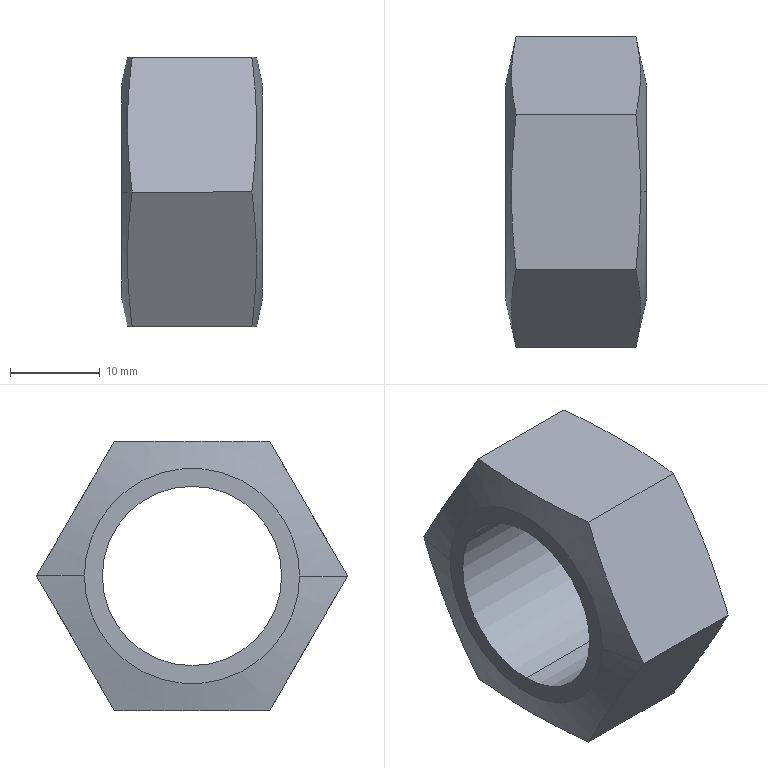Part | SolidWorks | features BaseBody 1 | 1 solid | 14 faces | box 15.7 x 34.641 x 30 mm | volume 7009 mm3 | plane 8 | cone 4 | cylinder 2 | commonest cylinder face diameters 20 x2
STEP:
#1=CARTESIAN_POINT('',(65.7,0.,-10.));
#2=VERTEX_POINT('',#1);
#3=CARTESIAN_POINT('',(65.7,0.,10.));
#4=VERTEX_POINT('',#3);
#5=CARTESIAN_POINT('',(65.7,0.,0.));
#6=DIRECTION('',(-1.,0.,0.));
#7=DIRECTION('',(0.,0.,1.));
#8=AXIS2_PLACEMENT_3D('',#5,#6,#7);
#9=CIRCLE('',#8,10.);
#10=EDGE_CURVE('',#2,#4,#9,.T.);
#11=ORIENTED_EDGE('',*,*,#10,.F.);
#12=CARTESIAN_POINT('',(50.,0.,-10.));
#13=VERTEX_POINT('',#12);
#14=CARTESIAN_POINT('',(50.,0.,-10.));
#15=DIRECTION('',(-1.,0.,0.));
#16=VECTOR('',#15,1000.);
#17=LINE('',#14,#16);
#18=EDGE_CURVE('',#2,#13,#17,.T.);
#19=ORIENTED_EDGE('',*,*,#18,.T.);
#20=CARTESIAN_POINT('',(50.,0.,10.));
#21=VERTEX_POINT('',#20);
#22=CARTESIAN_POINT('',(50.,0.,0.));
#23=DIRECTION('',(1.,0.,0.));
#24=DIRECTION('',(0.,0.,1.));
#25=AXIS2_PLACEMENT_3D('',#22,#23,#24);
#26=CIRCLE('',#25,10.);
#27=EDGE_CURVE('',#21,#13,#26,.T.);
#28=ORIENTED_EDGE('',*,*,#27,.F.);
#29=CARTESIAN_POINT('',(50.,0.,10.));
#30=DIRECTION('',(-1.,0.,0.));
#31=VECTOR('',#30,1000.);
#32=LINE('',#29,#31);
#33=EDGE_CURVE('',#4,#21,#32,.T.);
#34=ORIENTED_EDGE('',*,*,#33,.F.);
#35=EDGE_LOOP('',(#11,#19,#28,#34));
#36=FACE_OUTER_BOUND('',#35,.T.);
#37=CARTESIAN_POINT('',(50.,0.,0.));
#38=DIRECTION('',(-1.,0.,0.));
#39=DIRECTION('',(0.,0.,1.));
#40=AXIS2_PLACEMENT_3D('',#37,#38,#39);
#41=CYLINDRICAL_SURFACE('',#40,10.);
#42=ADVANCED_FACE('',(#36),#41,.F.);
#43=CARTESIAN_POINT('',(65.7,0.,-12.));
#44=VERTEX_POINT('',#43);
#45=CARTESIAN_POINT('',(65.7,0.,12.));
#46=VERTEX_POINT('',#45);
#47=CARTESIAN_POINT('',(65.7,0.,0.));
#48=DIRECTION('',(1.,0.,0.));
#49=DIRECTION('',(0.,0.,1.));
#50=AXIS2_PLACEMENT_3D('',#47,#48,#49);
#51=CIRCLE('',#50,12.);
#52=EDGE_CURVE('',#44,#46,#51,.T.);
#53=ORIENTED_EDGE('',*,*,#52,.F.);
#54=CARTESIAN_POINT('',(65.033,0.,-15.));
#55=VERTEX_POINT('',#54);
#56=CARTESIAN_POINT('',(64.511,0.,-17.352));
#57=DIRECTION('',(-0.2169,0.,-0.9762));
#58=VECTOR('',#57,1000.);
#59=LINE('',#56,#58);
#60=EDGE_CURVE('',#44,#55,#59,.T.);
#61=ORIENTED_EDGE('',*,*,#60,.T.);
#62=CARTESIAN_POINT('',(64.518,8.66,-15.));
#63=VERTEX_POINT('',#62);
#64=CARTESIAN_POINT('',(65.033,0.,-15.));
#65=CARTESIAN_POINT('',(65.033,1.448,-15.));
#66=CARTESIAN_POINT('',(64.986,2.894,-15.));
#67=CARTESIAN_POINT('',(64.808,5.781,-15.));
#68=CARTESIAN_POINT('',(64.678,7.221,-15.));
#69=CARTESIAN_POINT('',(64.518,8.66,-15.));
#70=B_SPLINE_CURVE_WITH_KNOTS('',3,(#64,#65,#66,#67,#68,#69),.UNSPECIFIED.,.F.,.F.,(4,2,4),(0.,0.004338,0.008676),.UNSPECIFIED.);
#71=EDGE_CURVE('',#55,#63,#70,.T.);
#72=ORIENTED_EDGE('',*,*,#71,.T.);
#73=CARTESIAN_POINT('',(64.518,17.321,-0.00000001));
#74=VERTEX_POINT('',#73);
#75=CARTESIAN_POINT('',(64.518,8.66,-15.));
#76=CARTESIAN_POINT('',(64.678,9.382,-13.75));
#77=CARTESIAN_POINT('',(64.808,10.104,-12.5));
#78=CARTESIAN_POINT('',(64.986,11.547,-10.));
#79=CARTESIAN_POINT('',(65.08,12.99,-7.5));
#80=CARTESIAN_POINT('',(64.986,14.434,-5.));
#81=CARTESIAN_POINT('',(64.808,15.877,-2.5));
#82=CARTESIAN_POINT('',(64.678,16.599,-1.25));
#83=CARTESIAN_POINT('',(64.518,17.321,-0.00000001));
#84=B_SPLINE_CURVE_WITH_KNOTS('',3,(#75,#76,#77,#78,#79,#80,#81,#82,#83),.UNSPECIFIED.,.F.,.F.,(4,2,1,2,4),(0.,0.00433,0.00866,0.01299,0.01732),.UNSPECIFIED.);
#85=EDGE_CURVE('',#63,#74,#84,.T.);
#86=ORIENTED_EDGE('',*,*,#85,.T.);
#87=CARTESIAN_POINT('',(64.518,8.66,15.));
#88=VERTEX_POINT('',#87);
#89=CARTESIAN_POINT('',(64.518,17.321,-0.00000001));
#90=CARTESIAN_POINT('',(64.678,16.599,1.25));
#91=CARTESIAN_POINT('',(64.808,15.877,2.5));
#92=CARTESIAN_POINT('',(64.986,14.434,5.));
#93=CARTESIAN_POINT('',(65.08,12.99,7.5));
#94=CARTESIAN_POINT('',(64.986,11.547,10.));
#95=CARTESIAN_POINT('',(64.808,10.104,12.5));
#96=CARTESIAN_POINT('',(64.678,9.382,13.75));
#97=CARTESIAN_POINT('',(64.518,8.66,15.));
#98=B_SPLINE_CURVE_WITH_KNOTS('',3,(#89,#90,#91,#92,#93,#94,#95,#96,#97),.UNSPECIFIED.,.F.,.F.,(4,2,1,2,4),(0.,0.00433,0.00866,0.01299,0.01732),.UNSPECIFIED.);
#99=EDGE_CURVE('',#74,#88,#98,.T.);
#100=ORIENTED_EDGE('',*,*,#99,.T.);
#101=CARTESIAN_POINT('',(65.033,0.,15.));
#102=VERTEX_POINT('',#101);
#103=CARTESIAN_POINT('',(64.518,8.66,15.));
#104=CARTESIAN_POINT('',(64.678,7.221,15.));
#105=CARTESIAN_POINT('',(64.808,5.781,15.));
#106=CARTESIAN_POINT('',(64.986,2.894,15.));
#107=CARTESIAN_POINT('',(65.033,1.448,15.));
#108=CARTESIAN_POINT('',(65.033,0.,15.));
#109=B_SPLINE_CURVE_WITH_KNOTS('',3,(#103,#104,#105,#106,#107,#108),.UNSPECIFIED.,.F.,.F.,(4,2,4),(0.,0.004338,0.008676),.UNSPECIFIED.);
#110=EDGE_CURVE('',#88,#102,#109,.T.);
#111=ORIENTED_EDGE('',*,*,#110,.T.);
#112=CARTESIAN_POINT('',(64.511,0.,17.352));
#113=DIRECTION('',(-0.2169,0.,0.9762));
#114=VECTOR('',#113,1000.);
#115=LINE('',#112,#114);
#116=EDGE_CURVE('',#46,#102,#115,.T.);
#117=ORIENTED_EDGE('',*,*,#116,.F.);
#118=EDGE_LOOP('',(#53,#61,#72,#86,#100,#111,#117));
#119=FACE_OUTER_BOUND('',#118,.T.);
#120=CARTESIAN_POINT('',(64.511,0.,0.));
#121=DIRECTION('',(-1.,0.,0.));
#122=DIRECTION('',(0.,0.,1.));
#123=AXIS2_PLACEMENT_3D('',#120,#121,#122);
#124=CONICAL_SURFACE('',#123,17.352,1.352);
#125=ADVANCED_FACE('',(#119),#124,.T.);
#126=CARTESIAN_POINT('',(50.,-12.,0.));
#127=VERTEX_POINT('',#126);
#128=CARTESIAN_POINT('',(50.,12.,0.));
#129=VERTEX_POINT('',#128);
#130=CARTESIAN_POINT('',(50.,0.,0.));
#131=DIRECTION('',(-1.,0.,0.));
#132=DIRECTION('',(0.,1.,0.));
#133=AXIS2_PLACEMENT_3D('',#130,#131,#132);
#134=CIRCLE('',#133,12.);
#135=EDGE_CURVE('',#127,#129,#134,.T.);
#136=ORIENTED_EDGE('',*,*,#135,.F.);
#137=CARTESIAN_POINT('',(51.182,-17.321,-0.000000021));
#138=VERTEX_POINT('',#137);
#139=CARTESIAN_POINT('',(51.189,-17.352,0.));
#140=DIRECTION('',(0.2169,-0.9762,0.));
#141=VECTOR('',#140,1000.);
#142=LINE('',#139,#141);
#143=EDGE_CURVE('',#127,#138,#142,.T.);
#144=ORIENTED_EDGE('',*,*,#143,.T.);
#145=CARTESIAN_POINT('',(51.182,-8.66,15.));
#146=VERTEX_POINT('',#145);
#147=CARTESIAN_POINT('',(51.182,-17.321,-0.000000021));
#148=CARTESIAN_POINT('',(51.022,-16.599,1.25));
#149=CARTESIAN_POINT('',(50.892,-15.877,2.5));
#150=CARTESIAN_POINT('',(50.714,-14.434,5.));
#151=CARTESIAN_POINT('',(50.62,-12.99,7.5));
#152=CARTESIAN_POINT('',(50.714,-11.547,10.));
#153=CARTESIAN_POINT('',(50.892,-10.104,12.5));
#154=CARTESIAN_POINT('',(51.022,-9.382,13.75));
#155=CARTESIAN_POINT('',(51.182,-8.66,15.));
#156=B_SPLINE_CURVE_WITH_KNOTS('',3,(#147,#148,#149,#150,#151,#152,#153,#154,#155),.UNSPECIFIED.,.F.,.F.,(4,2,1,2,4),(0.,0.00433,0.00866,0.01299,0.01732),.UNSPECIFIED.);
#157=EDGE_CURVE('',#138,#146,#156,.T.);
#158=ORIENTED_EDGE('',*,*,#157,.T.);
#159=CARTESIAN_POINT('',(51.182,8.66,15.));
#160=VERTEX_POINT('',#159);
#161=CARTESIAN_POINT('',(51.182,-8.66,15.));
#162=CARTESIAN_POINT('',(51.022,-7.217,15.));
#163=CARTESIAN_POINT('',(50.892,-5.774,15.));
#164=CARTESIAN_POINT('',(50.714,-2.887,15.));
#165=CARTESIAN_POINT('',(50.62,-0.000000031,15.));
#166=CARTESIAN_POINT('',(50.714,2.887,15.));
#167=CARTESIAN_POINT('',(50.892,5.774,15.));
#168=CARTESIAN_POINT('',(51.022,7.217,15.));
#169=CARTESIAN_POINT('',(51.182,8.66,15.));
#170=B_SPLINE_CURVE_WITH_KNOTS('',3,(#161,#162,#163,#164,#165,#166,#167,#168,#169),.UNSPECIFIED.,.F.,.F.,(4,2,1,2,4),(0.,0.00433,0.00866,0.01299,0.01732),.UNSPECIFIED.);
#171=EDGE_CURVE('',#146,#160,#170,.T.);
#172=ORIENTED_EDGE('',*,*,#171,.T.);
#173=CARTESIAN_POINT('',(51.182,17.321,0.000000003));
#174=VERTEX_POINT('',#173);
#175=CARTESIAN_POINT('',(51.182,8.66,15.));
#176=CARTESIAN_POINT('',(51.022,9.382,13.75));
#177=CARTESIAN_POINT('',(50.892,10.104,12.5));
#178=CARTESIAN_POINT('',(50.714,11.547,10.));
#179=CARTESIAN_POINT('',(50.62,12.99,7.5));
#180=CARTESIAN_POINT('',(50.714,14.434,5.));
#181=CARTESIAN_POINT('',(50.892,15.877,2.5));
#182=CARTESIAN_POINT('',(51.022,16.599,1.25));
#183=CARTESIAN_POINT('',(51.182,17.321,0.000000003));
#184=B_SPLINE_CURVE_WITH_KNOTS('',3,(#175,#176,#177,#178,#179,#180,#181,#182,#183),.UNSPECIFIED.,.F.,.F.,(4,2,1,2,4),(0.,0.00433,0.00866,0.01299,0.01732),.UNSPECIFIED.);
#185=EDGE_CURVE('',#160,#174,#184,.T.);
#186=ORIENTED_EDGE('',*,*,#185,.T.);
#187=CARTESIAN_POINT('',(51.189,17.352,0.));
#188=DIRECTION('',(0.2169,0.9762,0.));
#189=VECTOR('',#188,1000.);
#190=LINE('',#187,#189);
#191=EDGE_CURVE('',#129,#174,#190,.T.);
#192=ORIENTED_EDGE('',*,*,#191,.F.);
#193=EDGE_LOOP('',(#136,#144,#158,#172,#186,#192));
#194=FACE_OUTER_BOUND('',#193,.T.);
#195=CARTESIAN_POINT('',(51.189,0.,0.));
#196=DIRECTION('',(1.,0.,0.));
#197=DIRECTION('',(0.,1.,0.));
#198=AXIS2_PLACEMENT_3D('',#195,#196,#197);
#199=CONICAL_SURFACE('',#198,17.352,1.352);
#200=ADVANCED_FACE('',(#194),#199,.T.);
#201=CARTESIAN_POINT('',(64.518,-8.66,15.));
#202=VERTEX_POINT('',#201);
#203=CARTESIAN_POINT('',(50.,-8.66,15.));
#204=DIRECTION('',(-1.,0.,0.));
#205=VECTOR('',#204,1000.);
#206=LINE('',#203,#205);
#207=EDGE_CURVE('',#202,#146,#206,.T.);
#208=ORIENTED_EDGE('',*,*,#207,.T.);
#209=ORIENTED_EDGE('',*,*,#157,.F.);
#210=CARTESIAN_POINT('',(64.518,-17.321,0.00000001));
#211=VERTEX_POINT('',#210);
#212=CARTESIAN_POINT('',(50.,-17.321,0.));
#213=DIRECTION('',(1.,0.,0.));
#214=VECTOR('',#213,1000.);
#215=LINE('',#212,#214);
#216=EDGE_CURVE('',#138,#211,#215,.T.);
#217=ORIENTED_EDGE('',*,*,#216,.T.);
#218=CARTESIAN_POINT('',(64.518,-8.66,15.));
#219=CARTESIAN_POINT('',(64.678,-9.382,13.75));
#220=CARTESIAN_POINT('',(64.808,-10.104,12.5));
#221=CARTESIAN_POINT('',(64.986,-11.547,10.));
#222=CARTESIAN_POINT('',(65.08,-12.99,7.5));
#223=CARTESIAN_POINT('',(64.986,-14.434,5.));
#224=CARTESIAN_POINT('',(64.808,-15.877,2.5));
#225=CARTESIAN_POINT('',(64.678,-16.599,1.25));
#226=CARTESIAN_POINT('',(64.518,-17.321,0.00000001));
#227=B_SPLINE_CURVE_WITH_KNOTS('',3,(#218,#219,#220,#221,#222,#223,#224,#225,#226),.UNSPECIFIED.,.F.,.F.,(4,2,1,2,4),(0.,0.00433,0.00866,0.01299,0.01732),.UNSPECIFIED.);
#228=EDGE_CURVE('',#202,#211,#227,.T.);
#229=ORIENTED_EDGE('',*,*,#228,.F.);
#230=EDGE_LOOP('',(#208,#209,#217,#229));
#231=FACE_OUTER_BOUND('',#230,.T.);
#232=CARTESIAN_POINT('',(50.,-8.66,15.));
#233=DIRECTION('',(0.,0.866,-0.5));
#234=DIRECTION('',(-1.,0.,0.));
#235=AXIS2_PLACEMENT_3D('',#232,#233,#234);
#236=PLANE('',#235);
#237=ADVANCED_FACE('',(#231),#236,.F.);
#238=ORIENTED_EDGE('',*,*,#216,.F.);
#239=CARTESIAN_POINT('',(51.182,-8.66,-15.));
#240=VERTEX_POINT('',#239);
#241=CARTESIAN_POINT('',(51.182,-8.66,-15.));
#242=CARTESIAN_POINT('',(51.022,-9.382,-13.75));
#243=CARTESIAN_POINT('',(50.892,-10.104,-12.5));
#244=CARTESIAN_POINT('',(50.714,-11.547,-10.));
#245=CARTESIAN_POINT('',(50.62,-12.99,-7.5));
#246=CARTESIAN_POINT('',(50.714,-14.434,-5.));
#247=CARTESIAN_POINT('',(50.892,-15.877,-2.5));
#248=CARTESIAN_POINT('',(51.022,-16.599,-1.25));
#249=CARTESIAN_POINT('',(51.182,-17.321,-0.000000021));
#250=B_SPLINE_CURVE_WITH_KNOTS('',3,(#241,#242,#243,#244,#245,#246,#247,#248,#249),.UNSPECIFIED.,.F.,.F.,(4,2,1,2,4),(0.,0.00433,0.00866,0.01299,0.01732),.UNSPECIFIED.);
#251=EDGE_CURVE('',#240,#138,#250,.T.);
#252=ORIENTED_EDGE('',*,*,#251,.F.);
#253=CARTESIAN_POINT('',(64.518,-8.66,-15.));
#254=VERTEX_POINT('',#253);
#255=CARTESIAN_POINT('',(50.,-8.66,-15.));
#256=DIRECTION('',(1.,0.,0.));
#257=VECTOR('',#256,1000.);
#258=LINE('',#255,#257);
#259=EDGE_CURVE('',#240,#254,#258,.T.);
#260=ORIENTED_EDGE('',*,*,#259,.T.);
#261=CARTESIAN_POINT('',(64.518,-17.321,0.00000001));
#262=CARTESIAN_POINT('',(64.678,-16.599,-1.25));
#263=CARTESIAN_POINT('',(64.808,-15.877,-2.5));
#264=CARTESIAN_POINT('',(64.986,-14.434,-5.));
#265=CARTESIAN_POINT('',(65.08,-12.99,-7.5));
#266=CARTESIAN_POINT('',(64.986,-11.547,-10.));
#267=CARTESIAN_POINT('',(64.808,-10.104,-12.5));
#268=CARTESIAN_POINT('',(64.678,-9.382,-13.75));
#269=CARTESIAN_POINT('',(64.518,-8.66,-15.));
#270=B_SPLINE_CURVE_WITH_KNOTS('',3,(#261,#262,#263,#264,#265,#266,#267,#268,#269),.UNSPECIFIED.,.F.,.F.,(4,2,1,2,4),(0.,0.00433,0.00866,0.01299,0.01732),.UNSPECIFIED.);
#271=EDGE_CURVE('',#211,#254,#270,.T.);
#272=ORIENTED_EDGE('',*,*,#271,.F.);
#273=EDGE_LOOP('',(#238,#252,#260,#272));
#274=FACE_OUTER_BOUND('',#273,.T.);
#275=CARTESIAN_POINT('',(50.,-17.321,0.));
#276=DIRECTION('',(0.,0.866,0.5));
#277=DIRECTION('',(1.,0.,0.));
#278=AXIS2_PLACEMENT_3D('',#275,#276,#277);
#279=PLANE('',#278);
#280=ADVANCED_FACE('',(#274),#279,.F.);
#281=ORIENTED_EDGE('',*,*,#259,.F.);
#282=CARTESIAN_POINT('',(51.182,8.66,-15.));
#283=VERTEX_POINT('',#282);
#284=CARTESIAN_POINT('',(51.182,8.66,-15.));
#285=CARTESIAN_POINT('',(51.022,7.217,-15.));
#286=CARTESIAN_POINT('',(50.892,5.774,-15.));
#287=CARTESIAN_POINT('',(50.714,2.887,-15.));
#288=CARTESIAN_POINT('',(50.62,0.000000031,-15.));
#289=CARTESIAN_POINT('',(50.714,-2.887,-15.));
#290=CARTESIAN_POINT('',(50.892,-5.774,-15.));
#291=CARTESIAN_POINT('',(51.022,-7.217,-15.));
#292=CARTESIAN_POINT('',(51.182,-8.66,-15.));
#293=B_SPLINE_CURVE_WITH_KNOTS('',3,(#284,#285,#286,#287,#288,#289,#290,#291,#292),.UNSPECIFIED.,.F.,.F.,(4,2,1,2,4),(0.,0.00433,0.00866,0.01299,0.01732),.UNSPECIFIED.);
#294=EDGE_CURVE('',#283,#240,#293,.T.);
#295=ORIENTED_EDGE('',*,*,#294,.F.);
#296=CARTESIAN_POINT('',(50.,8.66,-15.));
#297=DIRECTION('',(1.,0.,0.));
#298=VECTOR('',#297,1000.);
#299=LINE('',#296,#298);
#300=EDGE_CURVE('',#283,#63,#299,.T.);
#301=ORIENTED_EDGE('',*,*,#300,.T.);
#302=ORIENTED_EDGE('',*,*,#71,.F.);
#303=CARTESIAN_POINT('',(64.518,-8.66,-15.));
#304=CARTESIAN_POINT('',(64.678,-7.221,-15.));
#305=CARTESIAN_POINT('',(64.808,-5.781,-15.));
#306=CARTESIAN_POINT('',(64.986,-2.894,-15.));
#307=CARTESIAN_POINT('',(65.033,-1.448,-15.));
#308=CARTESIAN_POINT('',(65.033,0.,-15.));
#309=B_SPLINE_CURVE_WITH_KNOTS('',3,(#303,#304,#305,#306,#307,#308),.UNSPECIFIED.,.F.,.F.,(4,2,4),(-0.008676,-0.004338,0.),.UNSPECIFIED.);
#310=EDGE_CURVE('',#254,#55,#309,.T.);
#311=ORIENTED_EDGE('',*,*,#310,.F.);
#312=EDGE_LOOP('',(#281,#295,#301,#302,#311));
#313=FACE_OUTER_BOUND('',#312,.T.);
#314=CARTESIAN_POINT('',(50.,-8.66,-15.));
#315=DIRECTION('',(0.,0.,1.));
#316=DIRECTION('',(1.,0.,0.));
#317=AXIS2_PLACEMENT_3D('',#314,#315,#316);
#318=PLANE('',#317);
#319=ADVANCED_FACE('',(#313),#318,.F.);
#320=ORIENTED_EDGE('',*,*,#300,.F.);
#321=CARTESIAN_POINT('',(51.182,17.321,0.000000003));
#322=CARTESIAN_POINT('',(51.022,16.599,-1.25));
#323=CARTESIAN_POINT('',(50.892,15.877,-2.5));
#324=CARTESIAN_POINT('',(50.714,14.434,-5.));
#325=CARTESIAN_POINT('',(50.62,12.99,-7.5));
#326=CARTESIAN_POINT('',(50.714,11.547,-10.));
#327=CARTESIAN_POINT('',(50.892,10.104,-12.5));
#328=CARTESIAN_POINT('',(51.022,9.382,-13.75));
#329=CARTESIAN_POINT('',(51.182,8.66,-15.));
#330=B_SPLINE_CURVE_WITH_KNOTS('',3,(#321,#322,#323,#324,#325,#326,#327,#328,#329),.UNSPECIFIED.,.F.,.F.,(4,2,1,2,4),(0.,0.00433,0.00866,0.01299,0.01732),.UNSPECIFIED.);
#331=EDGE_CURVE('',#174,#283,#330,.T.);
#332=ORIENTED_EDGE('',*,*,#331,.F.);
#333=CARTESIAN_POINT('',(50.,17.321,0.));
#334=DIRECTION('',(1.,0.,0.));
#335=VECTOR('',#334,1000.);
#336=LINE('',#333,#335);
#337=EDGE_CURVE('',#174,#74,#336,.T.);
#338=ORIENTED_EDGE('',*,*,#337,.T.);
#339=ORIENTED_EDGE('',*,*,#85,.F.);
#340=EDGE_LOOP('',(#320,#332,#338,#339));
#341=FACE_OUTER_BOUND('',#340,.T.);
#342=CARTESIAN_POINT('',(50.,8.66,-15.));
#343=DIRECTION('',(0.,-0.866,0.5));
#344=DIRECTION('',(-1.,0.,0.));
#345=AXIS2_PLACEMENT_3D('',#342,#343,#344);
#346=PLANE('',#345);
#347=ADVANCED_FACE('',(#341),#346,.F.);
#348=ORIENTED_EDGE('',*,*,#337,.F.);
#349=ORIENTED_EDGE('',*,*,#185,.F.);
#350=CARTESIAN_POINT('',(50.,8.66,15.));
#351=DIRECTION('',(1.,0.,0.));
#352=VECTOR('',#351,1000.);
#353=LINE('',#350,#352);
#354=EDGE_CURVE('',#160,#88,#353,.T.);
#355=ORIENTED_EDGE('',*,*,#354,.T.);
#356=ORIENTED_EDGE('',*,*,#99,.F.);
#357=EDGE_LOOP('',(#348,#349,#355,#356));
#358=FACE_OUTER_BOUND('',#357,.T.);
#359=CARTESIAN_POINT('',(50.,17.321,0.));
#360=DIRECTION('',(0.,-0.866,-0.5));
#361=DIRECTION('',(0.,0.5,-0.866));
#362=AXIS2_PLACEMENT_3D('',#359,#360,#361);
#363=PLANE('',#362);
#364=ADVANCED_FACE('',(#358),#363,.F.);
#365=ORIENTED_EDGE('',*,*,#354,.F.);
#366=ORIENTED_EDGE('',*,*,#171,.F.);
#367=ORIENTED_EDGE('',*,*,#207,.F.);
#368=CARTESIAN_POINT('',(65.033,0.,15.));
#369=CARTESIAN_POINT('',(65.033,-1.448,15.));
#370=CARTESIAN_POINT('',(64.986,-2.894,15.));
#371=CARTESIAN_POINT('',(64.808,-5.781,15.));
#372=CARTESIAN_POINT('',(64.678,-7.221,15.));
#373=CARTESIAN_POINT('',(64.518,-8.66,15.));
#374=B_SPLINE_CURVE_WITH_KNOTS('',3,(#368,#369,#370,#371,#372,#373),.UNSPECIFIED.,.F.,.F.,(4,2,4),(0.008676,0.01301,0.01735),.UNSPECIFIED.);
#375=EDGE_CURVE('',#102,#202,#374,.T.);
#376=ORIENTED_EDGE('',*,*,#375,.F.);
#377=ORIENTED_EDGE('',*,*,#110,.F.);
#378=EDGE_LOOP('',(#365,#366,#367,#376,#377));
#379=FACE_OUTER_BOUND('',#378,.T.);
#380=CARTESIAN_POINT('',(50.,8.66,15.));
#381=DIRECTION('',(0.,0.,-1.));
#382=DIRECTION('',(0.,-1.,0.));
#383=AXIS2_PLACEMENT_3D('',#380,#381,#382);
#384=PLANE('',#383);
#385=ADVANCED_FACE('',(#379),#384,.F.);
#386=ORIENTED_EDGE('',*,*,#27,.T.);
#387=CARTESIAN_POINT('',(50.,0.,0.));
#388=DIRECTION('',(1.,0.,0.));
#389=DIRECTION('',(0.,0.,1.));
#390=AXIS2_PLACEMENT_3D('',#387,#388,#389);
#391=CIRCLE('',#390,10.);
#392=EDGE_CURVE('',#13,#21,#391,.T.);
#393=ORIENTED_EDGE('',*,*,#392,.T.);
#394=EDGE_LOOP('',(#386,#393));
#395=FACE_BOUND('',#394,.T.);
#396=CARTESIAN_POINT('',(50.,0.,0.));
#397=DIRECTION('',(-1.,0.,0.));
#398=DIRECTION('',(0.,1.,0.));
#399=AXIS2_PLACEMENT_3D('',#396,#397,#398);
#400=CIRCLE('',#399,12.);
#401=EDGE_CURVE('',#129,#127,#400,.T.);
#402=ORIENTED_EDGE('',*,*,#401,.T.);
#403=ORIENTED_EDGE('',*,*,#135,.T.);
#404=EDGE_LOOP('',(#402,#403));
#405=FACE_OUTER_BOUND('',#404,.T.);
#406=CARTESIAN_POINT('',(50.,0.,-6.));
#407=DIRECTION('',(-1.,0.,0.));
#408=DIRECTION('',(0.,1.,0.));
#409=AXIS2_PLACEMENT_3D('',#406,#407,#408);
#410=PLANE('',#409);
#411=ADVANCED_FACE('',(#395,#405),#410,.T.);
#412=CARTESIAN_POINT('',(65.7,0.,0.));
#413=DIRECTION('',(-1.,0.,0.));
#414=DIRECTION('',(0.,0.,1.));
#415=AXIS2_PLACEMENT_3D('',#412,#413,#414);
#416=CIRCLE('',#415,10.);
#417=EDGE_CURVE('',#4,#2,#416,.T.);
#418=ORIENTED_EDGE('',*,*,#417,.T.);
#419=ORIENTED_EDGE('',*,*,#10,.T.);
#420=EDGE_LOOP('',(#418,#419));
#421=FACE_BOUND('',#420,.T.);
#422=CARTESIAN_POINT('',(65.7,0.,0.));
#423=DIRECTION('',(1.,0.,0.));
#424=DIRECTION('',(0.,0.,1.));
#425=AXIS2_PLACEMENT_3D('',#422,#423,#424);
#426=CIRCLE('',#425,12.);
#427=EDGE_CURVE('',#46,#44,#426,.T.);
#428=ORIENTED_EDGE('',*,*,#427,.T.);
#429=ORIENTED_EDGE('',*,*,#52,.T.);
#430=EDGE_LOOP('',(#428,#429));
#431=FACE_OUTER_BOUND('',#430,.T.);
#432=CARTESIAN_POINT('',(65.7,0.,-6.));
#433=DIRECTION('',(1.,0.,0.));
#434=DIRECTION('',(0.,1.,0.));
#435=AXIS2_PLACEMENT_3D('',#432,#433,#434);
#436=PLANE('',#435);
#437=ADVANCED_FACE('',(#421,#431),#436,.T.);
#438=ORIENTED_EDGE('',*,*,#143,.F.);
#439=ORIENTED_EDGE('',*,*,#401,.F.);
#440=ORIENTED_EDGE('',*,*,#191,.T.);
#441=ORIENTED_EDGE('',*,*,#331,.T.);
#442=ORIENTED_EDGE('',*,*,#294,.T.);
#443=ORIENTED_EDGE('',*,*,#251,.T.);
#444=EDGE_LOOP('',(#438,#439,#440,#441,#442,#443));
#445=FACE_OUTER_BOUND('',#444,.T.);
#446=CARTESIAN_POINT('',(51.189,0.,0.));
#447=DIRECTION('',(1.,0.,0.));
#448=DIRECTION('',(0.,1.,0.));
#449=AXIS2_PLACEMENT_3D('',#446,#447,#448);
#450=CONICAL_SURFACE('',#449,17.352,1.352);
#451=ADVANCED_FACE('',(#445),#450,.T.);
#452=ORIENTED_EDGE('',*,*,#60,.F.);
#453=ORIENTED_EDGE('',*,*,#427,.F.);
#454=ORIENTED_EDGE('',*,*,#116,.T.);
#455=ORIENTED_EDGE('',*,*,#375,.T.);
#456=ORIENTED_EDGE('',*,*,#228,.T.);
#457=ORIENTED_EDGE('',*,*,#271,.T.);
#458=ORIENTED_EDGE('',*,*,#310,.T.);
#459=EDGE_LOOP('',(#452,#453,#454,#455,#456,#457,#458));
#460=FACE_OUTER_BOUND('',#459,.T.);
#461=CARTESIAN_POINT('',(64.511,0.,0.));
#462=DIRECTION('',(-1.,0.,0.));
#463=DIRECTION('',(0.,0.,1.));
#464=AXIS2_PLACEMENT_3D('',#461,#462,#463);
#465=CONICAL_SURFACE('',#464,17.352,1.352);
#466=ADVANCED_FACE('',(#460),#465,.T.);
#467=ORIENTED_EDGE('',*,*,#18,.F.);
#468=ORIENTED_EDGE('',*,*,#417,.F.);
#469=ORIENTED_EDGE('',*,*,#33,.T.);
#470=ORIENTED_EDGE('',*,*,#392,.F.);
#471=EDGE_LOOP('',(#467,#468,#469,#470));
#472=FACE_OUTER_BOUND('',#471,.T.);
#473=CARTESIAN_POINT('',(50.,0.,0.));
#474=DIRECTION('',(-1.,0.,0.));
#475=DIRECTION('',(0.,0.,1.));
#476=AXIS2_PLACEMENT_3D('',#473,#474,#475);
#477=CYLINDRICAL_SURFACE('',#476,10.);
#478=ADVANCED_FACE('',(#472),#477,.F.);
#479=CLOSED_SHELL('',(#42,#125,#200,#237,#280,#319,#347,#364,#385,#411,#437,#451,#466,#478));
#480=MANIFOLD_SOLID_BREP('',#479);
#481=CARTESIAN_POINT('',(0.,0.,0.));
#482=DIRECTION('',(0.,0.,1.));
#483=DIRECTION('',(1.,0.,0.));
#484=AXIS2_PLACEMENT_3D('',#481,#482,#483);
#485=(LENGTH_UNIT()NAMED_UNIT(*)SI_UNIT(.MILLI.,.METRE.));
#486=UNCERTAINTY_MEASURE_WITH_UNIT(LENGTH_MEASURE(0.00001),#485,'','');
#487=(NAMED_UNIT(*)PLANE_ANGLE_UNIT()SI_UNIT($,.RADIAN.));
#488=(NAMED_UNIT(*)SI_UNIT($,.STERADIAN.)SOLID_ANGLE_UNIT());
#489=(GEOMETRIC_REPRESENTATION_CONTEXT(3)GLOBAL_UNCERTAINTY_ASSIGNED_CONTEXT((#486))GLOBAL_UNIT_ASSIGNED_CONTEXT((#485,#487,#488))REPRESENTATION_CONTEXT('',''));
#490=ADVANCED_BREP_SHAPE_REPRESENTATION('',(#480,#484),#489);